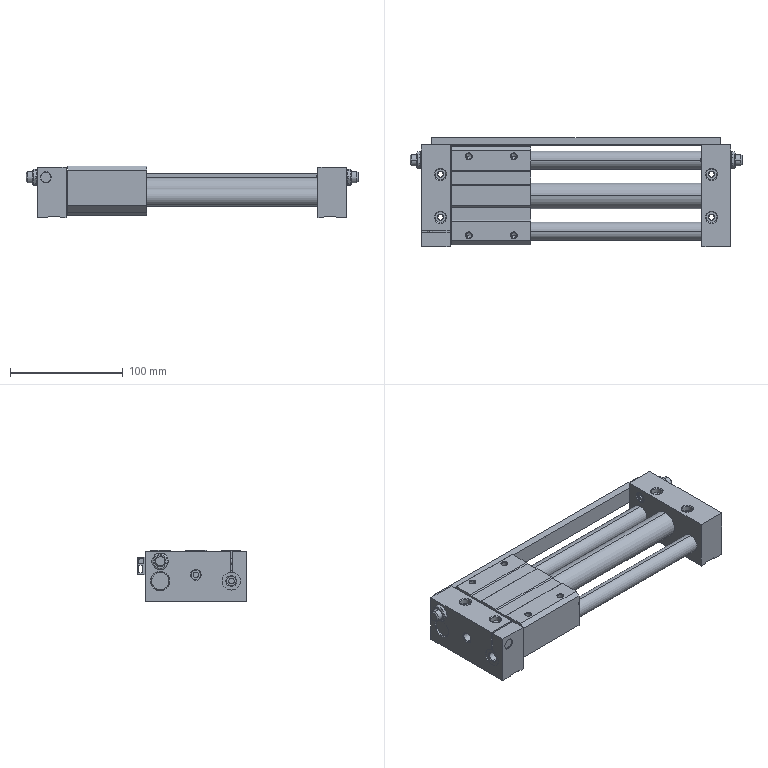Part | SolidWorks | features BaseBody 4, MoveCopyBody 1 | 4 solids | 435 faces | box 294 x 96.8 x 46 mm | volume 580391 mm3 | plane 165 | cylinder 156 | cone 106 | torus 8 | commonest cylinder face diameters 4.917 x16 16 x14 15 x12 3 x8 5 x8 5.5 x8